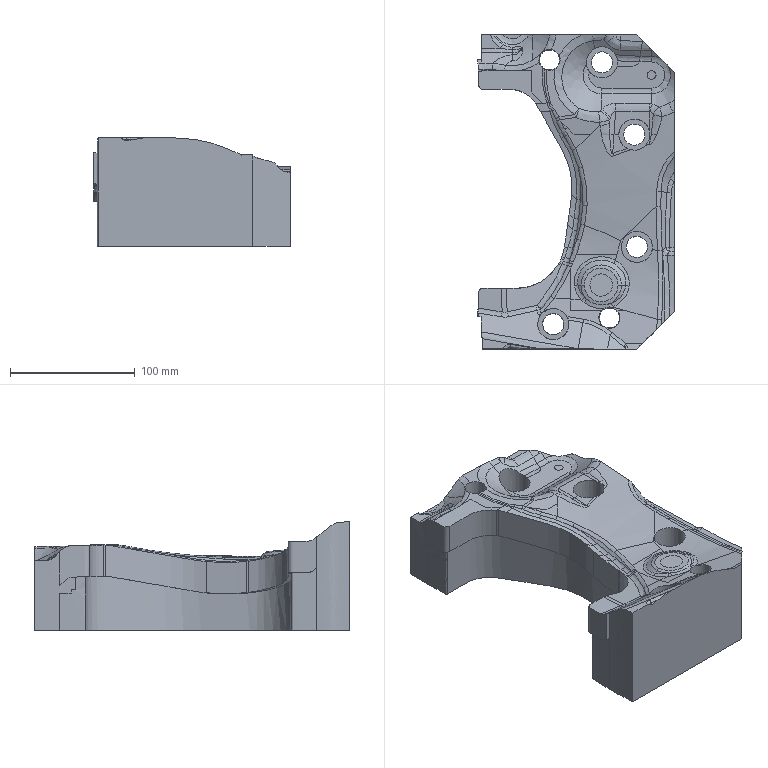Part | NX | features solid 2 | 1 solid | 257 faces | box 157.617 x 252.645 x 87.328 mm | volume 1626415 mm3 | spline 227 | plane 17 | cylinder 12 | sphere 1 | commonest cylinder face diameters 17 x6 25 x4 16 x2